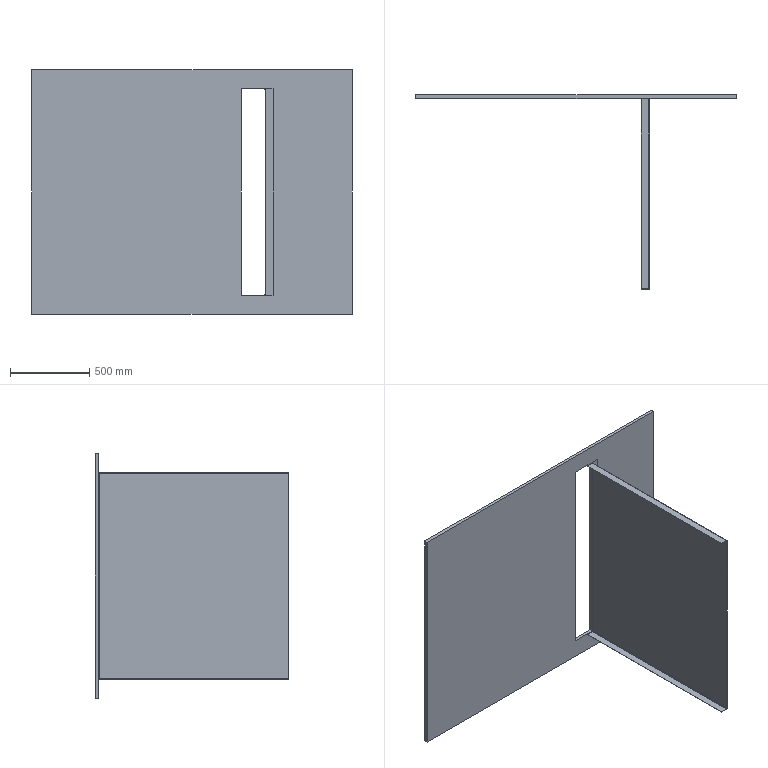Part | STEP file | 果蔬烘干机框架-107 | 2 solids | 42 faces | box 2020 x 1220 x 1540 mm | volume 60915530 mm3 | plane 36 | cylinder 6 | commonest cylinder face diameters 6 x3 9 x3
STEP:
#1=CARTESIAN_POINT('',(1010.,0.,770.));
#2=VERTEX_POINT('',#1);
#3=CARTESIAN_POINT('',(1010.,0.,-770.));
#4=VERTEX_POINT('',#3);
#5=CARTESIAN_POINT('',(1010.,0.,-770.));
#6=DIRECTION('',(0.,0.,-1.));
#7=VECTOR('',#6,1000.);
#8=LINE('',#5,#7);
#9=EDGE_CURVE('',#2,#4,#8,.T.);
#10=ORIENTED_EDGE('',*,*,#9,.T.);
#11=CARTESIAN_POINT('',(1010.,20.,-770.));
#12=VERTEX_POINT('',#11);
#13=CARTESIAN_POINT('',(1010.,20.,-770.));
#14=DIRECTION('',(0.,-1.,0.));
#15=VECTOR('',#14,1000.);
#16=LINE('',#13,#15);
#17=EDGE_CURVE('',#12,#4,#16,.T.);
#18=ORIENTED_EDGE('',*,*,#17,.F.);
#19=CARTESIAN_POINT('',(1010.,20.,770.));
#20=VERTEX_POINT('',#19);
#21=CARTESIAN_POINT('',(1010.,20.,-770.));
#22=DIRECTION('',(0.,0.,-1.));
#23=VECTOR('',#22,1000.);
#24=LINE('',#21,#23);
#25=EDGE_CURVE('',#20,#12,#24,.T.);
#26=ORIENTED_EDGE('',*,*,#25,.F.);
#27=CARTESIAN_POINT('',(1010.,20.,770.));
#28=DIRECTION('',(0.,-1.,0.));
#29=VECTOR('',#28,1000.);
#30=LINE('',#27,#29);
#31=EDGE_CURVE('',#20,#2,#30,.T.);
#32=ORIENTED_EDGE('',*,*,#31,.T.);
#33=EDGE_LOOP('',(#10,#18,#26,#32));
#34=FACE_OUTER_BOUND('',#33,.T.);
#35=CARTESIAN_POINT('',(1010.,20.,-770.));
#36=DIRECTION('',(-1.,0.,0.));
#37=DIRECTION('',(0.,0.,1.));
#38=AXIS2_PLACEMENT_3D('',#35,#36,#37);
#39=PLANE('',#38);
#40=ADVANCED_FACE('',(#34),#39,.F.);
#41=CARTESIAN_POINT('',(-1010.,0.,-770.));
#42=VERTEX_POINT('',#41);
#43=CARTESIAN_POINT('',(-1010.,0.,-770.));
#44=DIRECTION('',(-1.,0.,0.));
#45=VECTOR('',#44,1000.);
#46=LINE('',#43,#45);
#47=EDGE_CURVE('',#4,#42,#46,.T.);
#48=ORIENTED_EDGE('',*,*,#47,.T.);
#49=CARTESIAN_POINT('',(-1010.,20.,-770.));
#50=VERTEX_POINT('',#49);
#51=CARTESIAN_POINT('',(-1010.,20.,-770.));
#52=DIRECTION('',(0.,-1.,0.));
#53=VECTOR('',#52,1000.);
#54=LINE('',#51,#53);
#55=EDGE_CURVE('',#50,#42,#54,.T.);
#56=ORIENTED_EDGE('',*,*,#55,.F.);
#57=CARTESIAN_POINT('',(-1010.,20.,-770.));
#58=DIRECTION('',(-1.,0.,0.));
#59=VECTOR('',#58,1000.);
#60=LINE('',#57,#59);
#61=EDGE_CURVE('',#12,#50,#60,.T.);
#62=ORIENTED_EDGE('',*,*,#61,.F.);
#63=ORIENTED_EDGE('',*,*,#17,.T.);
#64=EDGE_LOOP('',(#48,#56,#62,#63));
#65=FACE_OUTER_BOUND('',#64,.T.);
#66=CARTESIAN_POINT('',(-1010.,20.,-770.));
#67=DIRECTION('',(0.,0.,1.));
#68=DIRECTION('',(1.,0.,0.));
#69=AXIS2_PLACEMENT_3D('',#66,#67,#68);
#70=PLANE('',#69);
#71=ADVANCED_FACE('',(#65),#70,.F.);
#72=CARTESIAN_POINT('',(-1010.,0.,770.));
#73=VERTEX_POINT('',#72);
#74=CARTESIAN_POINT('',(-1010.,0.,-770.));
#75=DIRECTION('',(0.,0.,1.));
#76=VECTOR('',#75,1000.);
#77=LINE('',#74,#76);
#78=EDGE_CURVE('',#42,#73,#77,.T.);
#79=ORIENTED_EDGE('',*,*,#78,.T.);
#80=CARTESIAN_POINT('',(-1010.,20.,770.));
#81=VERTEX_POINT('',#80);
#82=CARTESIAN_POINT('',(-1010.,20.,770.));
#83=DIRECTION('',(0.,-1.,0.));
#84=VECTOR('',#83,1000.);
#85=LINE('',#82,#84);
#86=EDGE_CURVE('',#81,#73,#85,.T.);
#87=ORIENTED_EDGE('',*,*,#86,.F.);
#88=CARTESIAN_POINT('',(-1010.,20.,-770.));
#89=DIRECTION('',(0.,0.,1.));
#90=VECTOR('',#89,1000.);
#91=LINE('',#88,#90);
#92=EDGE_CURVE('',#50,#81,#91,.T.);
#93=ORIENTED_EDGE('',*,*,#92,.F.);
#94=ORIENTED_EDGE('',*,*,#55,.T.);
#95=EDGE_LOOP('',(#79,#87,#93,#94));
#96=FACE_OUTER_BOUND('',#95,.T.);
#97=CARTESIAN_POINT('',(-1010.,20.,-770.));
#98=DIRECTION('',(1.,0.,0.));
#99=DIRECTION('',(0.,0.,-1.));
#100=AXIS2_PLACEMENT_3D('',#97,#98,#99);
#101=PLANE('',#100);
#102=ADVANCED_FACE('',(#96),#101,.F.);
#103=CARTESIAN_POINT('',(-1010.,0.,770.));
#104=DIRECTION('',(1.,0.,0.));
#105=VECTOR('',#104,1000.);
#106=LINE('',#103,#105);
#107=EDGE_CURVE('',#73,#2,#106,.T.);
#108=ORIENTED_EDGE('',*,*,#107,.T.);
#109=ORIENTED_EDGE('',*,*,#31,.F.);
#110=CARTESIAN_POINT('',(-1010.,20.,770.));
#111=DIRECTION('',(1.,0.,0.));
#112=VECTOR('',#111,1000.);
#113=LINE('',#110,#112);
#114=EDGE_CURVE('',#81,#20,#113,.T.);
#115=ORIENTED_EDGE('',*,*,#114,.F.);
#116=ORIENTED_EDGE('',*,*,#86,.T.);
#117=EDGE_LOOP('',(#108,#109,#115,#116));
#118=FACE_OUTER_BOUND('',#117,.T.);
#119=CARTESIAN_POINT('',(-1010.,20.,770.));
#120=DIRECTION('',(0.,0.,-1.));
#121=DIRECTION('',(-1.,0.,0.));
#122=AXIS2_PLACEMENT_3D('',#119,#120,#121);
#123=PLANE('',#122);
#124=ADVANCED_FACE('',(#118),#123,.F.);
#125=CARTESIAN_POINT('',(460.,20.,650.));
#126=VERTEX_POINT('',#125);
#127=CARTESIAN_POINT('',(460.,20.,-650.));
#128=VERTEX_POINT('',#127);
#129=CARTESIAN_POINT('',(460.,20.,-650.));
#130=DIRECTION('',(0.,0.,-1.));
#131=VECTOR('',#130,1000.);
#132=LINE('',#129,#131);
#133=EDGE_CURVE('',#126,#128,#132,.T.);
#134=ORIENTED_EDGE('',*,*,#133,.F.);
#135=CARTESIAN_POINT('',(310.,20.,650.));
#136=VERTEX_POINT('',#135);
#137=CARTESIAN_POINT('',(310.,20.,650.));
#138=DIRECTION('',(1.,0.,0.));
#139=VECTOR('',#138,1000.);
#140=LINE('',#137,#139);
#141=EDGE_CURVE('',#136,#126,#140,.T.);
#142=ORIENTED_EDGE('',*,*,#141,.F.);
#143=CARTESIAN_POINT('',(310.,20.,-650.));
#144=VERTEX_POINT('',#143);
#145=CARTESIAN_POINT('',(310.,20.,-650.));
#146=DIRECTION('',(0.,0.,1.));
#147=VECTOR('',#146,1000.);
#148=LINE('',#145,#147);
#149=EDGE_CURVE('',#144,#136,#148,.T.);
#150=ORIENTED_EDGE('',*,*,#149,.F.);
#151=CARTESIAN_POINT('',(310.,20.,-650.));
#152=DIRECTION('',(-1.,0.,0.));
#153=VECTOR('',#152,1000.);
#154=LINE('',#151,#153);
#155=EDGE_CURVE('',#128,#144,#154,.T.);
#156=ORIENTED_EDGE('',*,*,#155,.F.);
#157=EDGE_LOOP('',(#134,#142,#150,#156));
#158=FACE_BOUND('',#157,.T.);
#159=ORIENTED_EDGE('',*,*,#25,.T.);
#160=ORIENTED_EDGE('',*,*,#61,.T.);
#161=ORIENTED_EDGE('',*,*,#92,.T.);
#162=ORIENTED_EDGE('',*,*,#114,.T.);
#163=EDGE_LOOP('',(#159,#160,#161,#162));
#164=FACE_OUTER_BOUND('',#163,.T.);
#165=CARTESIAN_POINT('',(0.,20.,0.));
#166=DIRECTION('',(0.,1.,0.));
#167=DIRECTION('',(0.,0.,1.));
#168=AXIS2_PLACEMENT_3D('',#165,#166,#167);
#169=PLANE('',#168);
#170=ADVANCED_FACE('',(#158,#164),#169,.T.);
#171=CARTESIAN_POINT('',(310.,0.,650.));
#172=VERTEX_POINT('',#171);
#173=CARTESIAN_POINT('',(460.,0.,650.));
#174=VERTEX_POINT('',#173);
#175=CARTESIAN_POINT('',(310.,0.,650.));
#176=DIRECTION('',(1.,0.,0.));
#177=VECTOR('',#176,1000.);
#178=LINE('',#175,#177);
#179=EDGE_CURVE('',#172,#174,#178,.T.);
#180=ORIENTED_EDGE('',*,*,#179,.T.);
#181=CARTESIAN_POINT('',(460.,0.,-650.));
#182=VERTEX_POINT('',#181);
#183=CARTESIAN_POINT('',(460.,0.,-650.));
#184=DIRECTION('',(0.,0.,-1.));
#185=VECTOR('',#184,1000.);
#186=LINE('',#183,#185);
#187=EDGE_CURVE('',#174,#182,#186,.T.);
#188=ORIENTED_EDGE('',*,*,#187,.T.);
#189=CARTESIAN_POINT('',(310.,0.,-650.));
#190=VERTEX_POINT('',#189);
#191=CARTESIAN_POINT('',(310.,0.,-650.));
#192=DIRECTION('',(-1.,0.,0.));
#193=VECTOR('',#192,1000.);
#194=LINE('',#191,#193);
#195=EDGE_CURVE('',#182,#190,#194,.T.);
#196=ORIENTED_EDGE('',*,*,#195,.T.);
#197=CARTESIAN_POINT('',(310.,0.,-650.));
#198=DIRECTION('',(0.,0.,1.));
#199=VECTOR('',#198,1000.);
#200=LINE('',#197,#199);
#201=EDGE_CURVE('',#190,#172,#200,.T.);
#202=ORIENTED_EDGE('',*,*,#201,.T.);
#203=EDGE_LOOP('',(#180,#188,#196,#202));
#204=FACE_BOUND('',#203,.T.);
#205=ORIENTED_EDGE('',*,*,#9,.F.);
#206=ORIENTED_EDGE('',*,*,#107,.F.);
#207=ORIENTED_EDGE('',*,*,#78,.F.);
#208=ORIENTED_EDGE('',*,*,#47,.F.);
#209=EDGE_LOOP('',(#205,#206,#207,#208));
#210=FACE_OUTER_BOUND('',#209,.T.);
#211=CARTESIAN_POINT('',(0.,0.,0.));
#212=DIRECTION('',(0.,1.,0.));
#213=DIRECTION('',(0.,0.,1.));
#214=AXIS2_PLACEMENT_3D('',#211,#212,#213);
#215=PLANE('',#214);
#216=ADVANCED_FACE('',(#204,#210),#215,.F.);
#217=ORIENTED_EDGE('',*,*,#133,.T.);
#218=CARTESIAN_POINT('',(460.,0.,-650.));
#219=DIRECTION('',(0.,1.,0.));
#220=VECTOR('',#219,1000.);
#221=LINE('',#218,#220);
#222=EDGE_CURVE('',#182,#128,#221,.T.);
#223=ORIENTED_EDGE('',*,*,#222,.F.);
#224=ORIENTED_EDGE('',*,*,#187,.F.);
#225=CARTESIAN_POINT('',(460.,0.,650.));
#226=DIRECTION('',(0.,1.,0.));
#227=VECTOR('',#226,1000.);
#228=LINE('',#225,#227);
#229=EDGE_CURVE('',#174,#126,#228,.T.);
#230=ORIENTED_EDGE('',*,*,#229,.T.);
#231=EDGE_LOOP('',(#217,#223,#224,#230));
#232=FACE_OUTER_BOUND('',#231,.T.);
#233=CARTESIAN_POINT('',(460.,0.,-650.));
#234=DIRECTION('',(1.,0.,0.));
#235=DIRECTION('',(0.,0.,-1.));
#236=AXIS2_PLACEMENT_3D('',#233,#234,#235);
#237=PLANE('',#236);
#238=ADVANCED_FACE('',(#232),#237,.F.);
#239=ORIENTED_EDGE('',*,*,#141,.T.);
#240=ORIENTED_EDGE('',*,*,#229,.F.);
#241=ORIENTED_EDGE('',*,*,#179,.F.);
#242=CARTESIAN_POINT('',(310.,0.,650.));
#243=DIRECTION('',(0.,1.,0.));
#244=VECTOR('',#243,1000.);
#245=LINE('',#242,#244);
#246=EDGE_CURVE('',#172,#136,#245,.T.);
#247=ORIENTED_EDGE('',*,*,#246,.T.);
#248=EDGE_LOOP('',(#239,#240,#241,#247));
#249=FACE_OUTER_BOUND('',#248,.T.);
#250=CARTESIAN_POINT('',(310.,0.,650.));
#251=DIRECTION('',(0.,0.,1.));
#252=DIRECTION('',(1.,0.,0.));
#253=AXIS2_PLACEMENT_3D('',#250,#251,#252);
#254=PLANE('',#253);
#255=ADVANCED_FACE('',(#249),#254,.F.);
#256=ORIENTED_EDGE('',*,*,#149,.T.);
#257=ORIENTED_EDGE('',*,*,#246,.F.);
#258=ORIENTED_EDGE('',*,*,#201,.F.);
#259=CARTESIAN_POINT('',(310.,0.,-650.));
#260=DIRECTION('',(0.,1.,0.));
#261=VECTOR('',#260,1000.);
#262=LINE('',#259,#261);
#263=EDGE_CURVE('',#190,#144,#262,.T.);
#264=ORIENTED_EDGE('',*,*,#263,.T.);
#265=EDGE_LOOP('',(#256,#257,#258,#264));
#266=FACE_OUTER_BOUND('',#265,.T.);
#267=CARTESIAN_POINT('',(310.,0.,-650.));
#268=DIRECTION('',(-1.,0.,0.));
#269=DIRECTION('',(0.,0.,1.));
#270=AXIS2_PLACEMENT_3D('',#267,#268,#269);
#271=PLANE('',#270);
#272=ADVANCED_FACE('',(#266),#271,.F.);
#273=ORIENTED_EDGE('',*,*,#155,.T.);
#274=ORIENTED_EDGE('',*,*,#263,.F.);
#275=ORIENTED_EDGE('',*,*,#195,.F.);
#276=ORIENTED_EDGE('',*,*,#222,.T.);
#277=EDGE_LOOP('',(#273,#274,#275,#276));
#278=FACE_OUTER_BOUND('',#277,.T.);
#279=CARTESIAN_POINT('',(310.,0.,-650.));
#280=DIRECTION('',(0.,0.,-1.));
#281=DIRECTION('',(-1.,0.,0.));
#282=AXIS2_PLACEMENT_3D('',#279,#280,#281);
#283=PLANE('',#282);
#284=ADVANCED_FACE('',(#278),#283,.F.);
#285=CLOSED_SHELL('',(#40,#71,#102,#124,#170,#216,#238,#255,#272,#284));
#286=MANIFOLD_SOLID_BREP('',#285);
#287=CARTESIAN_POINT('',(464.5,-1.5,645.5));
#288=VERTEX_POINT('',#287);
#289=CARTESIAN_POINT('',(464.5,0.,645.5));
#290=VERTEX_POINT('',#289);
#291=CARTESIAN_POINT('',(464.5,-1.5,645.5));
#292=DIRECTION('',(0.,1.,0.));
#293=VECTOR('',#292,1000.);
#294=LINE('',#291,#293);
#295=EDGE_CURVE('',#288,#290,#294,.T.);
#296=ORIENTED_EDGE('',*,*,#295,.F.);
#297=CARTESIAN_POINT('',(464.5,-1.5,650.));
#298=VERTEX_POINT('',#297);
#299=CARTESIAN_POINT('',(464.5,-1.5,-650.));
#300=DIRECTION('',(0.,0.,1.));
#301=VECTOR('',#300,1000.);
#302=LINE('',#299,#301);
#303=EDGE_CURVE('',#288,#298,#302,.T.);
#304=ORIENTED_EDGE('',*,*,#303,.T.);
#305=CARTESIAN_POINT('',(464.5,0.,650.));
#306=VERTEX_POINT('',#305);
#307=CARTESIAN_POINT('',(464.5,-1.5,650.));
#308=DIRECTION('',(0.,1.,0.));
#309=VECTOR('',#308,1000.);
#310=LINE('',#307,#309);
#311=EDGE_CURVE('',#298,#306,#310,.T.);
#312=ORIENTED_EDGE('',*,*,#311,.T.);
#313=CARTESIAN_POINT('',(464.5,0.,-650.));
#314=DIRECTION('',(0.,0.,1.));
#315=VECTOR('',#314,1000.);
#316=LINE('',#313,#315);
#317=EDGE_CURVE('',#290,#306,#316,.T.);
#318=ORIENTED_EDGE('',*,*,#317,.F.);
#319=EDGE_LOOP('',(#296,#304,#312,#318));
#320=FACE_OUTER_BOUND('',#319,.T.);
#321=CARTESIAN_POINT('',(464.5,0.,0.));
#322=DIRECTION('',(-1.,0.,0.));
#323=DIRECTION('',(0.,0.,1.));
#324=AXIS2_PLACEMENT_3D('',#321,#322,#323);
#325=PLANE('',#324);
#326=ADVANCED_FACE('',(#320),#325,.T.);
#327=CARTESIAN_POINT('',(460.,-4.5,-645.5));
#328=VERTEX_POINT('',#327);
#329=CARTESIAN_POINT('',(460.,-4.5,645.5));
#330=VERTEX_POINT('',#329);
#331=CARTESIAN_POINT('',(460.,-4.5,650.));
#332=DIRECTION('',(0.,0.,1.));
#333=VECTOR('',#332,1000.);
#334=LINE('',#331,#333);
#335=EDGE_CURVE('',#328,#330,#334,.T.);
#336=ORIENTED_EDGE('',*,*,#335,.T.);
#337=CARTESIAN_POINT('',(464.5,-4.5,645.5));
#338=DIRECTION('',(0.,0.,-1.));
#339=DIRECTION('',(1.,0.,0.));
#340=AXIS2_PLACEMENT_3D('',#337,#338,#339);
#341=CIRCLE('',#340,4.5);
#342=EDGE_CURVE('',#330,#290,#341,.T.);
#343=ORIENTED_EDGE('',*,*,#342,.T.);
#344=CARTESIAN_POINT('',(464.5,0.,-645.5));
#345=VERTEX_POINT('',#344);
#346=CARTESIAN_POINT('',(464.5,0.,-650.));
#347=DIRECTION('',(0.,0.,1.));
#348=VECTOR('',#347,1000.);
#349=LINE('',#346,#348);
#350=EDGE_CURVE('',#345,#290,#349,.T.);
#351=ORIENTED_EDGE('',*,*,#350,.F.);
#352=CARTESIAN_POINT('',(464.5,-4.5,-645.5));
#353=DIRECTION('',(0.,0.,1.));
#354=DIRECTION('',(-1.,0.,0.));
#355=AXIS2_PLACEMENT_3D('',#352,#353,#354);
#356=CIRCLE('',#355,4.5);
#357=EDGE_CURVE('',#345,#328,#356,.T.);
#358=ORIENTED_EDGE('',*,*,#357,.T.);
#359=EDGE_LOOP('',(#336,#343,#351,#358));
#360=FACE_OUTER_BOUND('',#359,.T.);
#361=CARTESIAN_POINT('',(464.5,-4.5,-650.));
#362=DIRECTION('',(0.,0.,-1.));
#363=DIRECTION('',(-1.,0.,0.));
#364=AXIS2_PLACEMENT_3D('',#361,#362,#363);
#365=CYLINDRICAL_SURFACE('',#364,4.5);
#366=ADVANCED_FACE('',(#360),#365,.T.);
#367=CARTESIAN_POINT('',(461.5,-4.5,645.5));
#368=VERTEX_POINT('',#367);
#369=CARTESIAN_POINT('',(464.5,-4.5,645.5));
#370=DIRECTION('',(0.,0.,-1.));
#371=DIRECTION('',(1.,0.,0.));
#372=AXIS2_PLACEMENT_3D('',#369,#370,#371);
#373=CIRCLE('',#372,3.);
#374=EDGE_CURVE('',#368,#288,#373,.T.);
#375=ORIENTED_EDGE('',*,*,#374,.T.);
#376=ORIENTED_EDGE('',*,*,#295,.T.);
#377=ORIENTED_EDGE('',*,*,#342,.F.);
#378=CARTESIAN_POINT('',(460.,-4.5,645.5));
#379=DIRECTION('',(1.,0.,0.));
#380=VECTOR('',#379,1000.);
#381=LINE('',#378,#380);
#382=EDGE_CURVE('',#330,#368,#381,.T.);
#383=ORIENTED_EDGE('',*,*,#382,.T.);
#384=EDGE_LOOP('',(#375,#376,#377,#383));
#385=FACE_OUTER_BOUND('',#384,.T.);
#386=CARTESIAN_POINT('',(464.5,-4.5,645.5));
#387=DIRECTION('',(0.,0.,1.));
#388=DIRECTION('',(1.,0.,0.));
#389=AXIS2_PLACEMENT_3D('',#386,#387,#388);
#390=PLANE('',#389);
#391=ADVANCED_FACE('',(#385),#390,.T.);
#392=CARTESIAN_POINT('',(460.,-1200.,645.5));
#393=VERTEX_POINT('',#392);
#394=CARTESIAN_POINT('',(460.,-4.5,645.5));
#395=DIRECTION('',(0.,-1.,0.));
#396=VECTOR('',#395,1000.);
#397=LINE('',#394,#396);
#398=EDGE_CURVE('',#330,#393,#397,.T.);
#399=ORIENTED_EDGE('',*,*,#398,.F.);
#400=ORIENTED_EDGE('',*,*,#335,.F.);
#401=CARTESIAN_POINT('',(460.,-1200.,-645.5));
#402=VERTEX_POINT('',#401);
#403=CARTESIAN_POINT('',(460.,-1200.,-645.5));
#404=DIRECTION('',(0.,1.,0.));
#405=VECTOR('',#404,1000.);
#406=LINE('',#403,#405);
#407=EDGE_CURVE('',#402,#328,#406,.T.);
#408=ORIENTED_EDGE('',*,*,#407,.F.);
#409=CARTESIAN_POINT('',(460.,-1200.,0.));
#410=DIRECTION('',(0.,0.,1.));
#411=VECTOR('',#410,1000.);
#412=LINE('',#409,#411);
#413=EDGE_CURVE('',#402,#393,#412,.T.);
#414=ORIENTED_EDGE('',*,*,#413,.T.);
#415=EDGE_LOOP('',(#399,#400,#408,#414));
#416=FACE_OUTER_BOUND('',#415,.T.);
#417=CARTESIAN_POINT('',(460.,0.,0.));
#418=DIRECTION('',(1.,0.,0.));
#419=DIRECTION('',(0.,1.,0.));
#420=AXIS2_PLACEMENT_3D('',#417,#418,#419);
#421=PLANE('',#420);
#422=ADVANCED_FACE('',(#416),#421,.F.);
#423=CARTESIAN_POINT('',(461.5,-4.5,-645.5));
#424=VERTEX_POINT('',#423);
#425=CARTESIAN_POINT('',(461.5,-4.5,650.));
#426=DIRECTION('',(0.,0.,-1.));
#427=VECTOR('',#426,1000.);
#428=LINE('',#425,#427);
#429=EDGE_CURVE('',#368,#424,#428,.T.);
#430=ORIENTED_EDGE('',*,*,#429,.F.);
#431=CARTESIAN_POINT('',(461.5,-1200.,645.5));
#432=VERTEX_POINT('',#431);
#433=CARTESIAN_POINT('',(461.5,-4.5,645.5));
#434=DIRECTION('',(0.,-1.,0.));
#435=VECTOR('',#434,1000.);
#436=LINE('',#433,#435);
#437=EDGE_CURVE('',#368,#432,#436,.T.);
#438=ORIENTED_EDGE('',*,*,#437,.T.);
#439=CARTESIAN_POINT('',(461.5,-1200.,-645.5));
#440=VERTEX_POINT('',#439);
#441=CARTESIAN_POINT('',(461.5,-1200.,650.));
#442=DIRECTION('',(0.,0.,1.));
#443=VECTOR('',#442,1000.);
#444=LINE('',#441,#443);
#445=EDGE_CURVE('',#440,#432,#444,.T.);
#446=ORIENTED_EDGE('',*,*,#445,.F.);
#447=CARTESIAN_POINT('',(461.5,-1200.,-645.5));
#448=DIRECTION('',(0.,1.,0.));
#449=VECTOR('',#448,1000.);
#450=LINE('',#447,#449);
#451=EDGE_CURVE('',#440,#424,#450,.T.);
#452=ORIENTED_EDGE('',*,*,#451,.T.);
#453=EDGE_LOOP('',(#430,#438,#446,#452));
#454=FACE_OUTER_BOUND('',#453,.T.);
#455=CARTESIAN_POINT('',(461.5,0.,0.));
#456=DIRECTION('',(1.,0.,0.));
#457=DIRECTION('',(0.,1.,0.));
#458=AXIS2_PLACEMENT_3D('',#455,#456,#457);
#459=PLANE('',#458);
#460=ADVANCED_FACE('',(#454),#459,.T.);
#461=CARTESIAN_POINT('',(460.,-1200.,645.5));
#462=DIRECTION('',(1.,0.,0.));
#463=VECTOR('',#462,1000.);
#464=LINE('',#461,#463);
#465=EDGE_CURVE('',#393,#432,#464,.T.);
#466=ORIENTED_EDGE('',*,*,#465,.F.);
#467=ORIENTED_EDGE('',*,*,#413,.F.);
#468=CARTESIAN_POINT('',(460.,-1200.,-645.5));
#469=DIRECTION('',(1.,0.,0.));
#470=VECTOR('',#469,1000.);
#471=LINE('',#468,#470);
#472=EDGE_CURVE('',#402,#440,#471,.T.);
#473=ORIENTED_EDGE('',*,*,#472,.T.);
#474=ORIENTED_EDGE('',*,*,#445,.T.);
#475=EDGE_LOOP('',(#466,#467,#473,#474));
#476=FACE_OUTER_BOUND('',#475,.T.);
#477=CARTESIAN_POINT('',(460.,-1200.,650.));
#478=DIRECTION('',(0.,1.,0.));
#479=DIRECTION('',(-1.,0.,0.));
#480=AXIS2_PLACEMENT_3D('',#477,#478,#479);
#481=PLANE('',#480);
#482=ADVANCED_FACE('',(#476),#481,.F.);
#483=CARTESIAN_POINT('',(464.5,-1.5,-645.5));
#484=VERTEX_POINT('',#483);
#485=CARTESIAN_POINT('',(464.5,0.,-645.5));
#486=DIRECTION('',(0.,-1.,0.));
#487=VECTOR('',#486,1000.);
#488=LINE('',#485,#487);
#489=EDGE_CURVE('',#345,#484,#488,.T.);
#490=ORIENTED_EDGE('',*,*,#489,.F.);
#491=CARTESIAN_POINT('',(464.5,0.,-650.));
#492=VERTEX_POINT('',#491);
#493=CARTESIAN_POINT('',(464.5,0.,-650.));
#494=DIRECTION('',(0.,0.,1.));
#495=VECTOR('',#494,1000.);
#496=LINE('',#493,#495);
#497=EDGE_CURVE('',#492,#345,#496,.T.);
#498=ORIENTED_EDGE('',*,*,#497,.F.);
#499=CARTESIAN_POINT('',(464.5,-1.5,-650.));
#500=VERTEX_POINT('',#499);
#501=CARTESIAN_POINT('',(464.5,-1.5,-650.));
#502=DIRECTION('',(0.,1.,0.));
#503=VECTOR('',#502,1000.);
#504=LINE('',#501,#503);
#505=EDGE_CURVE('',#500,#492,#504,.T.);
#506=ORIENTED_EDGE('',*,*,#505,.F.);
#507=CARTESIAN_POINT('',(464.5,-1.5,-650.));
#508=DIRECTION('',(0.,0.,1.));
#509=VECTOR('',#508,1000.);
#510=LINE('',#507,#509);
#511=EDGE_CURVE('',#500,#484,#510,.T.);
#512=ORIENTED_EDGE('',*,*,#511,.T.);
#513=EDGE_LOOP('',(#490,#498,#506,#512));
#514=FACE_OUTER_BOUND('',#513,.T.);
#515=CARTESIAN_POINT('',(464.5,0.,0.));
#516=DIRECTION('',(1.,0.,0.));
#517=DIRECTION('',(0.,0.,-1.));
#518=AXIS2_PLACEMENT_3D('',#515,#516,#517);
#519=PLANE('',#518);
#520=ADVANCED_FACE('',(#514),#519,.F.);
#521=ORIENTED_EDGE('',*,*,#505,.T.);
#522=CARTESIAN_POINT('',(510.,0.,-650.));
#523=VERTEX_POINT('',#522);
#524=CARTESIAN_POINT('',(460.,0.,-650.));
#525=DIRECTION('',(1.,0.,0.));
#526=VECTOR('',#525,1000.);
#527=LINE('',#524,#526);
#528=EDGE_CURVE('',#492,#523,#527,.T.);
#529=ORIENTED_EDGE('',*,*,#528,.T.);
#530=CARTESIAN_POINT('',(510.,-1.5,-650.));
#531=VERTEX_POINT('',#530);
#532=CARTESIAN_POINT('',(510.,-1.5,-650.));
#533=DIRECTION('',(0.,1.,0.));
#534=VECTOR('',#533,1000.);
#535=LINE('',#532,#534);
#536=EDGE_CURVE('',#531,#523,#535,.T.);
#537=ORIENTED_EDGE('',*,*,#536,.F.);
#538=CARTESIAN_POINT('',(460.,-1.5,-650.));
#539=DIRECTION('',(1.,0.,0.));
#540=VECTOR('',#539,1000.);
#541=LINE('',#538,#540);
#542=EDGE_CURVE('',#500,#531,#541,.T.);
#543=ORIENTED_EDGE('',*,*,#542,.F.);
#544=EDGE_LOOP('',(#521,#529,#537,#543));
#545=FACE_OUTER_BOUND('',#544,.T.);
#546=CARTESIAN_POINT('',(460.,-1.5,-650.));
#547=DIRECTION('',(0.,0.,1.));
#548=DIRECTION('',(1.,0.,0.));
#549=AXIS2_PLACEMENT_3D('',#546,#547,#548);
#550=PLANE('',#549);
#551=ADVANCED_FACE('',(#545),#550,.F.);
#552=ORIENTED_EDGE('',*,*,#311,.F.);
#553=CARTESIAN_POINT('',(510.,-1.5,650.));
#554=VERTEX_POINT('',#553);
#555=CARTESIAN_POINT('',(460.,-1.5,650.));
#556=DIRECTION('',(-1.,0.,0.));
#557=VECTOR('',#556,1000.);
#558=LINE('',#555,#557);
#559=EDGE_CURVE('',#554,#298,#558,.T.);
#560=ORIENTED_EDGE('',*,*,#559,.F.);
#561=CARTESIAN_POINT('',(510.,0.,650.));
#562=VERTEX_POINT('',#561);
#563=CARTESIAN_POINT('',(510.,-1.5,650.));
#564=DIRECTION('',(0.,1.,0.));
#565=VECTOR('',#564,1000.);
#566=LINE('',#563,#565);
#567=EDGE_CURVE('',#554,#562,#566,.T.);
#568=ORIENTED_EDGE('',*,*,#567,.T.);
#569=CARTESIAN_POINT('',(460.,0.,650.));
#570=DIRECTION('',(-1.,0.,0.));
#571=VECTOR('',#570,1000.);
#572=LINE('',#569,#571);
#573=EDGE_CURVE('',#562,#306,#572,.T.);
#574=ORIENTED_EDGE('',*,*,#573,.T.);
#575=EDGE_LOOP('',(#552,#560,#568,#574));
#576=FACE_OUTER_BOUND('',#575,.T.);
#577=CARTESIAN_POINT('',(460.,-1.5,650.));
#578=DIRECTION('',(0.,0.,-1.));
#579=DIRECTION('',(-1.,0.,0.));
#580=AXIS2_PLACEMENT_3D('',#577,#578,#579);
#581=PLANE('',#580);
#582=ADVANCED_FACE('',(#576),#581,.F.);
#583=ORIENTED_EDGE('',*,*,#559,.T.);
#584=ORIENTED_EDGE('',*,*,#303,.F.);
#585=CARTESIAN_POINT('',(464.5,-1.5,-650.));
#586=DIRECTION('',(0.,0.,1.));
#587=VECTOR('',#586,1000.);
#588=LINE('',#585,#587);
#589=EDGE_CURVE('',#484,#288,#588,.T.);
#590=ORIENTED_EDGE('',*,*,#589,.F.);
#591=ORIENTED_EDGE('',*,*,#511,.F.);
#592=ORIENTED_EDGE('',*,*,#542,.T.);
#593=CARTESIAN_POINT('',(510.,-1.5,650.));
#594=DIRECTION('',(0.,0.,1.));
#595=VECTOR('',#594,1000.);
#596=LINE('',#593,#595);
#597=EDGE_CURVE('',#531,#554,#596,.T.);
#598=ORIENTED_EDGE('',*,*,#597,.T.);
#599=EDGE_LOOP('',(#583,#584,#590,#591,#592,#598));
#600=FACE_OUTER_BOUND('',#599,.T.);
#601=CARTESIAN_POINT('',(0.,-1.5,0.));
#602=DIRECTION('',(0.,-1.,0.));
#603=DIRECTION('',(0.,0.,-1.));
#604=AXIS2_PLACEMENT_3D('',#601,#602,#603);
#605=PLANE('',#604);
#606=ADVANCED_FACE('',(#600),#605,.T.);
#607=ORIENTED_EDGE('',*,*,#497,.T.);
#608=ORIENTED_EDGE('',*,*,#350,.T.);
#609=ORIENTED_EDGE('',*,*,#317,.T.);
#610=ORIENTED_EDGE('',*,*,#573,.F.);
#611=CARTESIAN_POINT('',(510.,0.,650.));
#612=DIRECTION('',(0.,0.,1.));
#613=VECTOR('',#612,1000.);
#614=LINE('',#611,#613);
#615=EDGE_CURVE('',#523,#562,#614,.T.);
#616=ORIENTED_EDGE('',*,*,#615,.F.);
#617=ORIENTED_EDGE('',*,*,#528,.F.);
#618=EDGE_LOOP('',(#607,#608,#609,#610,#616,#617));
#619=FACE_OUTER_BOUND('',#618,.T.);
#620=CARTESIAN_POINT('',(0.,0.,0.));
#621=DIRECTION('',(0.,-1.,0.));
#622=DIRECTION('',(0.,0.,-1.));
#623=AXIS2_PLACEMENT_3D('',#620,#621,#622);
#624=PLANE('',#623);
#625=ADVANCED_FACE('',(#619),#624,.F.);
#626=ORIENTED_EDGE('',*,*,#615,.T.);
#627=ORIENTED_EDGE('',*,*,#567,.F.);
#628=ORIENTED_EDGE('',*,*,#597,.F.);
#629=ORIENTED_EDGE('',*,*,#536,.T.);
#630=EDGE_LOOP('',(#626,#627,#628,#629));
#631=FACE_OUTER_BOUND('',#630,.T.);
#632=CARTESIAN_POINT('',(510.,-1.5,650.));
#633=DIRECTION('',(-1.,0.,0.));
#634=DIRECTION('',(0.,0.,1.));
#635=AXIS2_PLACEMENT_3D('',#632,#633,#634);
#636=PLANE('',#635);
#637=ADVANCED_FACE('',(#631),#636,.F.);
#638=ORIENTED_EDGE('',*,*,#357,.F.);
#639=ORIENTED_EDGE('',*,*,#489,.T.);
#640=CARTESIAN_POINT('',(464.5,-4.5,-645.5));
#641=DIRECTION('',(0.,0.,1.));
#642=DIRECTION('',(-1.,0.,0.));
#643=AXIS2_PLACEMENT_3D('',#640,#641,#642);
#644=CIRCLE('',#643,3.);
#645=EDGE_CURVE('',#484,#424,#644,.T.);
#646=ORIENTED_EDGE('',*,*,#645,.T.);
#647=CARTESIAN_POINT('',(460.,-4.5,-645.5));
#648=DIRECTION('',(1.,0.,0.));
#649=VECTOR('',#648,1000.);
#650=LINE('',#647,#649);
#651=EDGE_CURVE('',#328,#424,#650,.T.);
#652=ORIENTED_EDGE('',*,*,#651,.F.);
#653=EDGE_LOOP('',(#638,#639,#646,#652));
#654=FACE_OUTER_BOUND('',#653,.T.);
#655=CARTESIAN_POINT('',(464.5,-4.5,-645.5));
#656=DIRECTION('',(0.,0.,-1.));
#657=DIRECTION('',(-1.,0.,0.));
#658=AXIS2_PLACEMENT_3D('',#655,#656,#657);
#659=PLANE('',#658);
#660=ADVANCED_FACE('',(#654),#659,.T.);
#661=ORIENTED_EDGE('',*,*,#374,.F.);
#662=ORIENTED_EDGE('',*,*,#429,.T.);
#663=ORIENTED_EDGE('',*,*,#645,.F.);
#664=ORIENTED_EDGE('',*,*,#589,.T.);
#665=EDGE_LOOP('',(#661,#662,#663,#664));
#666=FACE_OUTER_BOUND('',#665,.T.);
#667=CARTESIAN_POINT('',(464.5,-4.5,-650.));
#668=DIRECTION('',(0.,0.,-1.));
#669=DIRECTION('',(-1.,0.,0.));
#670=AXIS2_PLACEMENT_3D('',#667,#668,#669);
#671=CYLINDRICAL_SURFACE('',#670,3.);
#672=ADVANCED_FACE('',(#666),#671,.F.);
#673=CARTESIAN_POINT('',(457.,-4.5,-648.5));
#674=VERTEX_POINT('',#673);
#675=CARTESIAN_POINT('',(457.,-4.5,-650.));
#676=VERTEX_POINT('',#675);
#677=CARTESIAN_POINT('',(457.,-4.5,-650.));
#678=DIRECTION('',(0.,0.,-1.));
#679=VECTOR('',#678,1000.);
#680=LINE('',#677,#679);
#681=EDGE_CURVE('',#674,#676,#680,.T.);
#682=ORIENTED_EDGE('',*,*,#681,.F.);
#683=CARTESIAN_POINT('',(457.,-4.5,-645.5));
#684=DIRECTION('',(0.,1.,0.));
#685=DIRECTION('',(0.,0.,-1.));
#686=AXIS2_PLACEMENT_3D('',#683,#684,#685);
#687=CIRCLE('',#686,3.);
#688=EDGE_CURVE('',#328,#674,#687,.T.);
#689=ORIENTED_EDGE('',*,*,#688,.F.);
#690=ORIENTED_EDGE('',*,*,#651,.T.);
#691=CARTESIAN_POINT('',(457.,-4.5,-645.5));
#692=DIRECTION('',(0.,1.,0.));
#693=DIRECTION('',(0.,0.,-1.));
#694=AXIS2_PLACEMENT_3D('',#691,#692,#693);
#695=CIRCLE('',#694,4.5);
#696=EDGE_CURVE('',#424,#676,#695,.T.);
#697=ORIENTED_EDGE('',*,*,#696,.T.);
#698=EDGE_LOOP('',(#682,#689,#690,#697));
#699=FACE_OUTER_BOUND('',#698,.T.);
#700=CARTESIAN_POINT('',(457.,-4.5,-645.5));
#701=DIRECTION('',(0.,1.,0.));
#702=DIRECTION('',(0.,0.,1.));
#703=AXIS2_PLACEMENT_3D('',#700,#701,#702);
#704=PLANE('',#703);
#705=ADVANCED_FACE('',(#699),#704,.T.);
#706=CARTESIAN_POINT('',(457.,-1200.,-648.5));
#707=VERTEX_POINT('',#706);
#708=CARTESIAN_POINT('',(457.,-1200.,-645.5));
#709=DIRECTION('',(0.,-1.,0.));
#710=DIRECTION('',(0.,0.,-1.));
#711=AXIS2_PLACEMENT_3D('',#708,#709,#710);
#712=CIRCLE('',#711,3.);
#713=EDGE_CURVE('',#707,#402,#712,.T.);
#714=ORIENTED_EDGE('',*,*,#713,.F.);
#715=CARTESIAN_POINT('',(457.,-1200.,-650.));
#716=VERTEX_POINT('',#715);
#717=CARTESIAN_POINT('',(457.,-1200.,-648.5));
#718=DIRECTION('',(0.,0.,-1.));
#719=VECTOR('',#718,1000.);
#720=LINE('',#717,#719);
#721=EDGE_CURVE('',#707,#716,#720,.T.);
#722=ORIENTED_EDGE('',*,*,#721,.T.);
#723=CARTESIAN_POINT('',(457.,-1200.,-645.5));
#724=DIRECTION('',(0.,-1.,0.));
#725=DIRECTION('',(0.,0.,-1.));
#726=AXIS2_PLACEMENT_3D('',#723,#724,#725);
#727=CIRCLE('',#726,4.5);
#728=EDGE_CURVE('',#716,#440,#727,.T.);
#729=ORIENTED_EDGE('',*,*,#728,.T.);
#730=ORIENTED_EDGE('',*,*,#472,.F.);
#731=EDGE_LOOP('',(#714,#722,#729,#730));
#732=FACE_OUTER_BOUND('',#731,.T.);
#733=CARTESIAN_POINT('',(457.,-1200.,-645.5));
#734=DIRECTION('',(0.,1.,0.));
#735=DIRECTION('',(0.,0.,1.));
#736=AXIS2_PLACEMENT_3D('',#733,#734,#735);
#737=PLANE('',#736);
#738=ADVANCED_FACE('',(#732),#737,.F.);
#739=ORIENTED_EDGE('',*,*,#451,.F.);
#740=ORIENTED_EDGE('',*,*,#728,.F.);
#741=CARTESIAN_POINT('',(457.,-4.5,-650.));
#742=DIRECTION('',(0.,1.,0.));
#743=VECTOR('',#742,1000.);
#744=LINE('',#741,#743);
#745=EDGE_CURVE('',#716,#676,#744,.T.);
#746=ORIENTED_EDGE('',*,*,#745,.T.);
#747=ORIENTED_EDGE('',*,*,#696,.F.);
#748=EDGE_LOOP('',(#739,#740,#746,#747));
#749=FACE_OUTER_BOUND('',#748,.T.);
#750=CARTESIAN_POINT('',(457.,-1200.,-645.5));
#751=DIRECTION('',(0.,-1.,0.));
#752=DIRECTION('',(0.,0.,-1.));
#753=AXIS2_PLACEMENT_3D('',#750,#751,#752);
#754=CYLINDRICAL_SURFACE('',#753,4.5);
#755=ADVANCED_FACE('',(#749),#754,.T.);
#756=ORIENTED_EDGE('',*,*,#407,.T.);
#757=ORIENTED_EDGE('',*,*,#688,.T.);
#758=CARTESIAN_POINT('',(457.,-4.5,-648.5));
#759=DIRECTION('',(0.,-1.,0.));
#760=VECTOR('',#759,1000.);
#761=LINE('',#758,#760);
#762=EDGE_CURVE('',#674,#707,#761,.T.);
#763=ORIENTED_EDGE('',*,*,#762,.T.);
#764=ORIENTED_EDGE('',*,*,#713,.T.);
#765=EDGE_LOOP('',(#756,#757,#763,#764));
#766=FACE_OUTER_BOUND('',#765,.T.);
#767=CARTESIAN_POINT('',(457.,-1200.,-645.5));
#768=DIRECTION('',(0.,-1.,0.));
#769=DIRECTION('',(0.,0.,-1.));
#770=AXIS2_PLACEMENT_3D('',#767,#768,#769);
#771=CYLINDRICAL_SURFACE('',#770,3.);
#772=ADVANCED_FACE('',(#766),#771,.F.);
#773=ORIENTED_EDGE('',*,*,#681,.T.);
#774=CARTESIAN_POINT('',(411.5,-4.5,-650.));
#775=VERTEX_POINT('',#774);
#776=CARTESIAN_POINT('',(0.,-4.5,-650.));
#777=DIRECTION('',(1.,0.,0.));
#778=VECTOR('',#777,1000.);
#779=LINE('',#776,#778);
#780=EDGE_CURVE('',#775,#676,#779,.T.);
#781=ORIENTED_EDGE('',*,*,#780,.F.);
#782=CARTESIAN_POINT('',(411.5,-4.5,-648.5));
#783=VERTEX_POINT('',#782);
#784=CARTESIAN_POINT('',(411.5,-4.5,-650.));
#785=DIRECTION('',(0.,0.,1.));
#786=VECTOR('',#785,1000.);
#787=LINE('',#784,#786);
#788=EDGE_CURVE('',#775,#783,#787,.T.);
#789=ORIENTED_EDGE('',*,*,#788,.T.);
#790=CARTESIAN_POINT('',(460.,-4.5,-648.5));
#791=DIRECTION('',(1.,0.,0.));
#792=VECTOR('',#791,1000.);
#793=LINE('',#790,#792);
#794=EDGE_CURVE('',#783,#674,#793,.T.);
#795=ORIENTED_EDGE('',*,*,#794,.T.);
#796=EDGE_LOOP('',(#773,#781,#789,#795));
#797=FACE_OUTER_BOUND('',#796,.T.);
#798=CARTESIAN_POINT('',(460.,-4.5,-650.));
#799=DIRECTION('',(0.,-1.,0.));
#800=DIRECTION('',(1.,0.,0.));
#801=AXIS2_PLACEMENT_3D('',#798,#799,#800);
#802=PLANE('',#801);
#803=ADVANCED_FACE('',(#797),#802,.F.);
#804=ORIENTED_EDGE('',*,*,#721,.F.);
#805=CARTESIAN_POINT('',(411.5,-1200.,-648.5));
#806=VERTEX_POINT('',#805);
#807=CARTESIAN_POINT('',(411.5,-1200.,-648.5));
#808=DIRECTION('',(-1.,0.,0.));
#809=VECTOR('',#808,1000.);
#810=LINE('',#807,#809);
#811=EDGE_CURVE('',#707,#806,#810,.T.);
#812=ORIENTED_EDGE('',*,*,#811,.T.);
#813=CARTESIAN_POINT('',(411.5,-1200.,-650.));
#814=VERTEX_POINT('',#813);
#815=CARTESIAN_POINT('',(411.5,-1200.,-650.));
#816=DIRECTION('',(0.,0.,1.));
#817=VECTOR('',#816,1000.);
#818=LINE('',#815,#817);
#819=EDGE_CURVE('',#814,#806,#818,.T.);
#820=ORIENTED_EDGE('',*,*,#819,.F.);
#821=CARTESIAN_POINT('',(0.,-1200.,-650.));
#822=DIRECTION('',(-1.,0.,0.));
#823=VECTOR('',#822,1000.);
#824=LINE('',#821,#823);
#825=EDGE_CURVE('',#716,#814,#824,.T.);
#826=ORIENTED_EDGE('',*,*,#825,.F.);
#827=EDGE_LOOP('',(#804,#812,#820,#826));
#828=FACE_OUTER_BOUND('',#827,.T.);
#829=CARTESIAN_POINT('',(411.5,-1200.,-650.));
#830=DIRECTION('',(0.,1.,0.));
#831=DIRECTION('',(-1.,0.,0.));
#832=AXIS2_PLACEMENT_3D('',#829,#830,#831);
#833=PLANE('',#832);
#834=ADVANCED_FACE('',(#828),#833,.F.);
#835=ORIENTED_EDGE('',*,*,#745,.F.);
#836=ORIENTED_EDGE('',*,*,#825,.T.);
#837=CARTESIAN_POINT('',(411.5,0.,-650.));
#838=DIRECTION('',(0.,1.,0.));
#839=VECTOR('',#838,1000.);
#840=LINE('',#837,#839);
#841=EDGE_CURVE('',#814,#775,#840,.T.);
#842=ORIENTED_EDGE('',*,*,#841,.T.);
#843=ORIENTED_EDGE('',*,*,#780,.T.);
#844=EDGE_LOOP('',(#835,#836,#842,#843));
#845=FACE_OUTER_BOUND('',#844,.T.);
#846=CARTESIAN_POINT('',(0.,0.,-650.));
#847=DIRECTION('',(0.,0.,1.));
#848=DIRECTION('',(1.,0.,0.));
#849=AXIS2_PLACEMENT_3D('',#846,#847,#848);
#850=PLANE('',#849);
#851=ADVANCED_FACE('',(#845),#850,.F.);
#852=ORIENTED_EDGE('',*,*,#811,.F.);
#853=ORIENTED_EDGE('',*,*,#762,.F.);
#854=ORIENTED_EDGE('',*,*,#794,.F.);
#855=CARTESIAN_POINT('',(411.5,-4.5,-648.5));
#856=DIRECTION('',(0.,1.,0.));
#857=VECTOR('',#856,1000.);
#858=LINE('',#855,#857);
#859=EDGE_CURVE('',#806,#783,#858,.T.);
#860=ORIENTED_EDGE('',*,*,#859,.F.);
#861=EDGE_LOOP('',(#852,#853,#854,#860));
#862=FACE_OUTER_BOUND('',#861,.T.);
#863=CARTESIAN_POINT('',(0.,0.,-648.5));
#864=DIRECTION('',(0.,0.,1.));
#865=DIRECTION('',(1.,0.,0.));
#866=AXIS2_PLACEMENT_3D('',#863,#864,#865);
#867=PLANE('',#866);
#868=ADVANCED_FACE('',(#862),#867,.T.);
#869=ORIENTED_EDGE('',*,*,#859,.T.);
#870=ORIENTED_EDGE('',*,*,#788,.F.);
#871=ORIENTED_EDGE('',*,*,#841,.F.);
#872=ORIENTED_EDGE('',*,*,#819,.T.);
#873=EDGE_LOOP('',(#869,#870,#871,#872));
#874=FACE_OUTER_BOUND('',#873,.T.);
#875=CARTESIAN_POINT('',(411.5,-4.5,-650.));
#876=DIRECTION('',(1.,0.,0.));
#877=DIRECTION('',(0.,0.,-1.));
#878=AXIS2_PLACEMENT_3D('',#875,#876,#877);
#879=PLANE('',#878);
#880=ADVANCED_FACE('',(#874),#879,.F.);
#881=CARTESIAN_POINT('',(457.,-1200.,648.5));
#882=VERTEX_POINT('',#881);
#883=CARTESIAN_POINT('',(457.,-1200.,650.));
#884=VERTEX_POINT('',#883);
#885=CARTESIAN_POINT('',(457.,-1200.,650.));
#886=DIRECTION('',(0.,0.,1.));
#887=VECTOR('',#886,1000.);
#888=LINE('',#885,#887);
#889=EDGE_CURVE('',#882,#884,#888,.T.);
#890=ORIENTED_EDGE('',*,*,#889,.F.);
#891=CARTESIAN_POINT('',(457.,-1200.,645.5));
#892=DIRECTION('',(0.,-1.,0.));
#893=DIRECTION('',(0.,0.,1.));
#894=AXIS2_PLACEMENT_3D('',#891,#892,#893);
#895=CIRCLE('',#894,3.);
#896=EDGE_CURVE('',#393,#882,#895,.T.);
#897=ORIENTED_EDGE('',*,*,#896,.F.);
#898=ORIENTED_EDGE('',*,*,#465,.T.);
#899=CARTESIAN_POINT('',(457.,-1200.,645.5));
#900=DIRECTION('',(0.,-1.,0.));
#901=DIRECTION('',(0.,0.,1.));
#902=AXIS2_PLACEMENT_3D('',#899,#900,#901);
#903=CIRCLE('',#902,4.5);
#904=EDGE_CURVE('',#432,#884,#903,.T.);
#905=ORIENTED_EDGE('',*,*,#904,.T.);
#906=EDGE_LOOP('',(#890,#897,#898,#905));
#907=FACE_OUTER_BOUND('',#906,.T.);
#908=CARTESIAN_POINT('',(457.,-1200.,645.5));
#909=DIRECTION('',(0.,-1.,0.));
#910=DIRECTION('',(0.,0.,-1.));
#911=AXIS2_PLACEMENT_3D('',#908,#909,#910);
#912=PLANE('',#911);
#913=ADVANCED_FACE('',(#907),#912,.T.);
#914=CARTESIAN_POINT('',(457.,-4.5,648.5));
#915=VERTEX_POINT('',#914);
#916=CARTESIAN_POINT('',(457.,-4.5,645.5));
#917=DIRECTION('',(0.,1.,0.));
#918=DIRECTION('',(0.,0.,1.));
#919=AXIS2_PLACEMENT_3D('',#916,#917,#918);
#920=CIRCLE('',#919,3.);
#921=EDGE_CURVE('',#915,#330,#920,.T.);
#922=ORIENTED_EDGE('',*,*,#921,.F.);
#923=CARTESIAN_POINT('',(457.,-4.5,650.));
#924=VERTEX_POINT('',#923);
#925=CARTESIAN_POINT('',(457.,-4.5,648.5));
#926=DIRECTION('',(0.,0.,1.));
#927=VECTOR('',#926,1000.);
#928=LINE('',#925,#927);
#929=EDGE_CURVE('',#915,#924,#928,.T.);
#930=ORIENTED_EDGE('',*,*,#929,.T.);
#931=CARTESIAN_POINT('',(457.,-4.5,645.5));
#932=DIRECTION('',(0.,1.,0.));
#933=DIRECTION('',(0.,0.,1.));
#934=AXIS2_PLACEMENT_3D('',#931,#932,#933);
#935=CIRCLE('',#934,4.5);
#936=EDGE_CURVE('',#924,#368,#935,.T.);
#937=ORIENTED_EDGE('',*,*,#936,.T.);
#938=ORIENTED_EDGE('',*,*,#382,.F.);
#939=EDGE_LOOP('',(#922,#930,#937,#938));
#940=FACE_OUTER_BOUND('',#939,.T.);
#941=CARTESIAN_POINT('',(457.,-4.5,645.5));
#942=DIRECTION('',(0.,-1.,0.));
#943=DIRECTION('',(0.,0.,-1.));
#944=AXIS2_PLACEMENT_3D('',#941,#942,#943);
#945=PLANE('',#944);
#946=ADVANCED_FACE('',(#940),#945,.F.);
#947=ORIENTED_EDGE('',*,*,#437,.F.);
#948=ORIENTED_EDGE('',*,*,#936,.F.);
#949=CARTESIAN_POINT('',(457.,-1200.,650.));
#950=DIRECTION('',(0.,-1.,0.));
#951=VECTOR('',#950,1000.);
#952=LINE('',#949,#951);
#953=EDGE_CURVE('',#924,#884,#952,.T.);
#954=ORIENTED_EDGE('',*,*,#953,.T.);
#955=ORIENTED_EDGE('',*,*,#904,.F.);
#956=EDGE_LOOP('',(#947,#948,#954,#955));
#957=FACE_OUTER_BOUND('',#956,.T.);
#958=CARTESIAN_POINT('',(457.,-4.5,645.5));
#959=DIRECTION('',(0.,1.,0.));
#960=DIRECTION('',(0.,0.,1.));
#961=AXIS2_PLACEMENT_3D('',#958,#959,#960);
#962=CYLINDRICAL_SURFACE('',#961,4.5);
#963=ADVANCED_FACE('',(#957),#962,.T.);
#964=ORIENTED_EDGE('',*,*,#398,.T.);
#965=ORIENTED_EDGE('',*,*,#896,.T.);
#966=CARTESIAN_POINT('',(457.,-1200.,648.5));
#967=DIRECTION('',(0.,1.,0.));
#968=VECTOR('',#967,1000.);
#969=LINE('',#966,#968);
#970=EDGE_CURVE('',#882,#915,#969,.T.);
#971=ORIENTED_EDGE('',*,*,#970,.T.);
#972=ORIENTED_EDGE('',*,*,#921,.T.);
#973=EDGE_LOOP('',(#964,#965,#971,#972));
#974=FACE_OUTER_BOUND('',#973,.T.);
#975=CARTESIAN_POINT('',(457.,-4.5,645.5));
#976=DIRECTION('',(0.,1.,0.));
#977=DIRECTION('',(0.,0.,1.));
#978=AXIS2_PLACEMENT_3D('',#975,#976,#977);
#979=CYLINDRICAL_SURFACE('',#978,3.);
#980=ADVANCED_FACE('',(#974),#979,.F.);
#981=ORIENTED_EDGE('',*,*,#889,.T.);
#982=CARTESIAN_POINT('',(411.5,-1200.,650.));
#983=VERTEX_POINT('',#982);
#984=CARTESIAN_POINT('',(0.,-1200.,650.));
#985=DIRECTION('',(1.,0.,0.));
#986=VECTOR('',#985,1000.);
#987=LINE('',#984,#986);
#988=EDGE_CURVE('',#983,#884,#987,.T.);
#989=ORIENTED_EDGE('',*,*,#988,.F.);
#990=CARTESIAN_POINT('',(411.5,-1200.,648.5));
#991=VERTEX_POINT('',#990);
#992=CARTESIAN_POINT('',(411.5,-1200.,650.));
#993=DIRECTION('',(0.,0.,-1.));
#994=VECTOR('',#993,1000.);
#995=LINE('',#992,#994);
#996=EDGE_CURVE('',#983,#991,#995,.T.);
#997=ORIENTED_EDGE('',*,*,#996,.T.);
#998=CARTESIAN_POINT('',(460.,-1200.,648.5));
#999=DIRECTION('',(1.,0.,0.));
#1000=VECTOR('',#999,1000.);
#1001=LINE('',#998,#1000);
#1002=EDGE_CURVE('',#991,#882,#1001,.T.);
#1003=ORIENTED_EDGE('',*,*,#1002,.T.);
#1004=EDGE_LOOP('',(#981,#989,#997,#1003));
#1005=FACE_OUTER_BOUND('',#1004,.T.);
#1006=CARTESIAN_POINT('',(460.,-1200.,650.));
#1007=DIRECTION('',(0.,1.,0.));
#1008=DIRECTION('',(-1.,0.,0.));
#1009=AXIS2_PLACEMENT_3D('',#1006,#1007,#1008);
#1010=PLANE('',#1009);
#1011=ADVANCED_FACE('',(#1005),#1010,.F.);
#1012=ORIENTED_EDGE('',*,*,#929,.F.);
#1013=CARTESIAN_POINT('',(411.5,-4.5,648.5));
#1014=VERTEX_POINT('',#1013);
#1015=CARTESIAN_POINT('',(411.5,-4.5,648.5));
#1016=DIRECTION('',(-1.,0.,0.));
#1017=VECTOR('',#1016,1000.);
#1018=LINE('',#1015,#1017);
#1019=EDGE_CURVE('',#915,#1014,#1018,.T.);
#1020=ORIENTED_EDGE('',*,*,#1019,.T.);
#1021=CARTESIAN_POINT('',(411.5,-4.5,650.));
#1022=VERTEX_POINT('',#1021);
#1023=CARTESIAN_POINT('',(411.5,-4.5,650.));
#1024=DIRECTION('',(0.,0.,-1.));
#1025=VECTOR('',#1024,1000.);
#1026=LINE('',#1023,#1025);
#1027=EDGE_CURVE('',#1022,#1014,#1026,.T.);
#1028=ORIENTED_EDGE('',*,*,#1027,.F.);
#1029=CARTESIAN_POINT('',(0.,-4.5,650.));
#1030=DIRECTION('',(-1.,0.,0.));
#1031=VECTOR('',#1030,1000.);
#1032=LINE('',#1029,#1031);
#1033=EDGE_CURVE('',#924,#1022,#1032,.T.);
#1034=ORIENTED_EDGE('',*,*,#1033,.F.);
#1035=EDGE_LOOP('',(#1012,#1020,#1028,#1034));
#1036=FACE_OUTER_BOUND('',#1035,.T.);
#1037=CARTESIAN_POINT('',(411.5,-4.5,650.));
#1038=DIRECTION('',(0.,-1.,0.));
#1039=DIRECTION('',(1.,0.,0.));
#1040=AXIS2_PLACEMENT_3D('',#1037,#1038,#1039);
#1041=PLANE('',#1040);
#1042=ADVANCED_FACE('',(#1036),#1041,.F.);
#1043=ORIENTED_EDGE('',*,*,#953,.F.);
#1044=ORIENTED_EDGE('',*,*,#1033,.T.);
#1045=CARTESIAN_POINT('',(411.5,0.,650.));
#1046=DIRECTION('',(0.,-1.,0.));
#1047=VECTOR('',#1046,1000.);
#1048=LINE('',#1045,#1047);
#1049=EDGE_CURVE('',#1022,#983,#1048,.T.);
#1050=ORIENTED_EDGE('',*,*,#1049,.T.);
#1051=ORIENTED_EDGE('',*,*,#988,.T.);
#1052=EDGE_LOOP('',(#1043,#1044,#1050,#1051));
#1053=FACE_OUTER_BOUND('',#1052,.T.);
#1054=CARTESIAN_POINT('',(0.,0.,650.));
#1055=DIRECTION('',(0.,0.,-1.));
#1056=DIRECTION('',(-1.,0.,0.));
#1057=AXIS2_PLACEMENT_3D('',#1054,#1055,#1056);
#1058=PLANE('',#1057);
#1059=ADVANCED_FACE('',(#1053),#1058,.F.);
#1060=ORIENTED_EDGE('',*,*,#1019,.F.);
#1061=ORIENTED_EDGE('',*,*,#970,.F.);
#1062=ORIENTED_EDGE('',*,*,#1002,.F.);
#1063=CARTESIAN_POINT('',(411.5,-1200.,648.5));
#1064=DIRECTION('',(0.,-1.,0.));
#1065=VECTOR('',#1064,1000.);
#1066=LINE('',#1063,#1065);
#1067=EDGE_CURVE('',#1014,#991,#1066,.T.);
#1068=ORIENTED_EDGE('',*,*,#1067,.F.);
#1069=EDGE_LOOP('',(#1060,#1061,#1062,#1068));
#1070=FACE_OUTER_BOUND('',#1069,.T.);
#1071=CARTESIAN_POINT('',(0.,0.,648.5));
#1072=DIRECTION('',(0.,0.,-1.));
#1073=DIRECTION('',(-1.,0.,0.));
#1074=AXIS2_PLACEMENT_3D('',#1071,#1072,#1073);
#1075=PLANE('',#1074);
#1076=ADVANCED_FACE('',(#1070),#1075,.T.);
#1077=ORIENTED_EDGE('',*,*,#1067,.T.);
#1078=ORIENTED_EDGE('',*,*,#996,.F.);
#1079=ORIENTED_EDGE('',*,*,#1049,.F.);
#1080=ORIENTED_EDGE('',*,*,#1027,.T.);
#1081=EDGE_LOOP('',(#1077,#1078,#1079,#1080));
#1082=FACE_OUTER_BOUND('',#1081,.T.);
#1083=CARTESIAN_POINT('',(411.5,-1200.,650.));
#1084=DIRECTION('',(1.,0.,0.));
#1085=DIRECTION('',(0.,0.,-1.));
#1086=AXIS2_PLACEMENT_3D('',#1083,#1084,#1085);
#1087=PLANE('',#1086);
#1088=ADVANCED_FACE('',(#1082),#1087,.F.);
#1089=CLOSED_SHELL('',(#326,#366,#391,#422,#460,#482,#520,#551,#582,#606,#625,#637,#660,#672,#705,#738,#755,#772,#803,#834,#851,#868,#880,#913,#946,#963,#980,#1011,#1042,#1059,#1076,#1088));
#1090=MANIFOLD_SOLID_BREP('',#1089);
#1091=CARTESIAN_POINT('',(0.,0.,0.));
#1092=DIRECTION('',(0.,0.,1.));
#1093=DIRECTION('',(1.,0.,0.));
#1094=AXIS2_PLACEMENT_3D('',#1091,#1092,#1093);
#1095=(LENGTH_UNIT()NAMED_UNIT(*)SI_UNIT(.MILLI.,.METRE.));
#1096=UNCERTAINTY_MEASURE_WITH_UNIT(LENGTH_MEASURE(0.00001),#1095,'','');
#1097=(NAMED_UNIT(*)PLANE_ANGLE_UNIT()SI_UNIT($,.RADIAN.));
#1098=(NAMED_UNIT(*)SI_UNIT($,.STERADIAN.)SOLID_ANGLE_UNIT());
#1099=(GEOMETRIC_REPRESENTATION_CONTEXT(3)GLOBAL_UNCERTAINTY_ASSIGNED_CONTEXT((#1096))GLOBAL_UNIT_ASSIGNED_CONTEXT((#1095,#1097,#1098))REPRESENTATION_CONTEXT('',''));
#1100=ADVANCED_BREP_SHAPE_REPRESENTATION('',(#286,#1090,#1094),#1099);